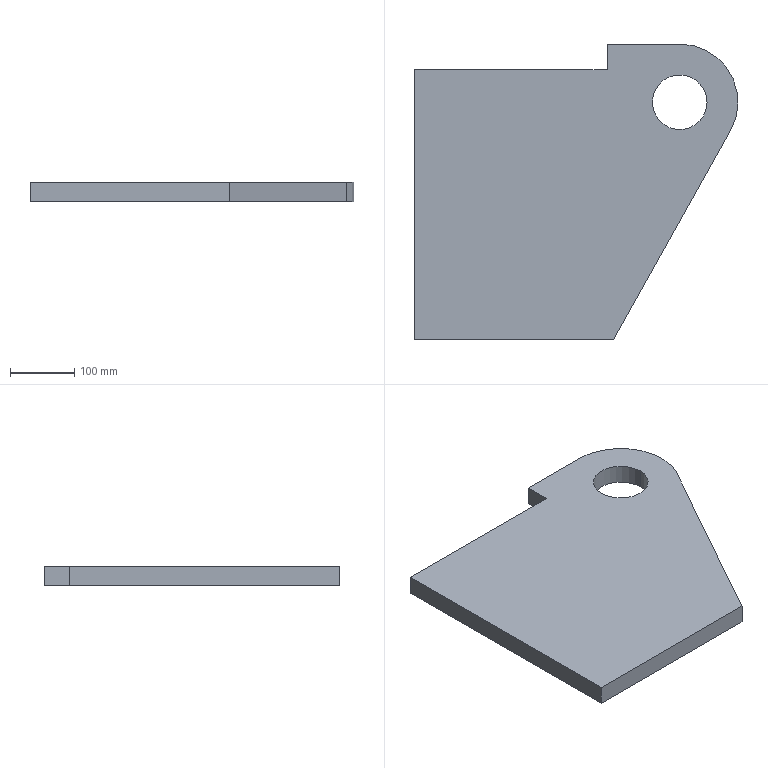Part | SolidWorks | features Extrusion 1 | 1 solid | 11 faces | box 503.5 x 460 x 30 mm | volume 5359945 mm3 | plane 8 | cylinder 3 | commonest cylinder face diameters 85 x2 181 x1
STEP:
#1=CARTESIAN_POINT('',(370.5,369.5,30.));
#2=VERTEX_POINT('',#1);
#3=CARTESIAN_POINT('',(455.5,369.5,30.));
#4=VERTEX_POINT('',#3);
#5=CARTESIAN_POINT('',(413.,369.5,30.));
#6=DIRECTION('',(0.,0.,1.));
#7=DIRECTION('',(1.,0.,0.));
#8=AXIS2_PLACEMENT_3D('',#5,#6,#7);
#9=CIRCLE('',#8,42.5);
#10=EDGE_CURVE('',#2,#4,#9,.T.);
#11=ORIENTED_EDGE('',*,*,#10,.T.);
#12=CARTESIAN_POINT('',(455.5,369.5,0.));
#13=VERTEX_POINT('',#12);
#14=CARTESIAN_POINT('',(455.5,369.5,30.));
#15=DIRECTION('',(0.,0.,-1.));
#16=VECTOR('',#15,1000.);
#17=LINE('',#14,#16);
#18=EDGE_CURVE('',#4,#13,#17,.T.);
#19=ORIENTED_EDGE('',*,*,#18,.T.);
#20=CARTESIAN_POINT('',(370.5,369.5,0.));
#21=VERTEX_POINT('',#20);
#22=CARTESIAN_POINT('',(413.,369.5,0.));
#23=DIRECTION('',(0.,0.,1.));
#24=DIRECTION('',(1.,0.,0.));
#25=AXIS2_PLACEMENT_3D('',#22,#23,#24);
#26=CIRCLE('',#25,42.5);
#27=EDGE_CURVE('',#21,#13,#26,.T.);
#28=ORIENTED_EDGE('',*,*,#27,.F.);
#29=CARTESIAN_POINT('',(370.5,369.5,30.));
#30=DIRECTION('',(0.,0.,-1.));
#31=VECTOR('',#30,1000.);
#32=LINE('',#29,#31);
#33=EDGE_CURVE('',#2,#21,#32,.T.);
#34=ORIENTED_EDGE('',*,*,#33,.F.);
#35=EDGE_LOOP('',(#11,#19,#28,#34));
#36=FACE_OUTER_BOUND('',#35,.T.);
#37=CARTESIAN_POINT('',(413.,369.5,30.));
#38=DIRECTION('',(0.,0.,-1.));
#39=DIRECTION('',(-1.,0.,0.));
#40=AXIS2_PLACEMENT_3D('',#37,#38,#39);
#41=CYLINDRICAL_SURFACE('',#40,42.5);
#42=ADVANCED_FACE('',(#36),#41,.F.);
#43=CARTESIAN_POINT('',(0.,0.,30.));
#44=VERTEX_POINT('',#43);
#45=CARTESIAN_POINT('',(310.,0.,30.));
#46=VERTEX_POINT('',#45);
#47=CARTESIAN_POINT('',(0.,0.,30.));
#48=DIRECTION('',(1.,0.,0.));
#49=VECTOR('',#48,1000.);
#50=LINE('',#47,#49);
#51=EDGE_CURVE('',#44,#46,#50,.T.);
#52=ORIENTED_EDGE('',*,*,#51,.T.);
#53=CARTESIAN_POINT('',(491.982,325.318,30.));
#54=VERTEX_POINT('',#53);
#55=CARTESIAN_POINT('',(310.,0.,30.));
#56=DIRECTION('',(0.4882,0.8727,0.));
#57=VECTOR('',#56,1000.);
#58=LINE('',#55,#57);
#59=EDGE_CURVE('',#46,#54,#58,.T.);
#60=ORIENTED_EDGE('',*,*,#59,.T.);
#61=CARTESIAN_POINT('',(413.,460.,30.));
#62=VERTEX_POINT('',#61);
#63=CARTESIAN_POINT('',(413.,369.5,30.));
#64=DIRECTION('',(0.,0.,1.));
#65=DIRECTION('',(1.,0.,0.));
#66=AXIS2_PLACEMENT_3D('',#63,#64,#65);
#67=CIRCLE('',#66,90.5);
#68=EDGE_CURVE('',#54,#62,#67,.T.);
#69=ORIENTED_EDGE('',*,*,#68,.T.);
#70=CARTESIAN_POINT('',(300.,460.,30.));
#71=VERTEX_POINT('',#70);
#72=CARTESIAN_POINT('',(300.,460.,30.));
#73=DIRECTION('',(-1.,0.,0.));
#74=VECTOR('',#73,1000.);
#75=LINE('',#72,#74);
#76=EDGE_CURVE('',#62,#71,#75,.T.);
#77=ORIENTED_EDGE('',*,*,#76,.T.);
#78=CARTESIAN_POINT('',(300.,420.,30.));
#79=VERTEX_POINT('',#78);
#80=CARTESIAN_POINT('',(300.,420.,30.));
#81=DIRECTION('',(0.,-1.,0.));
#82=VECTOR('',#81,1000.);
#83=LINE('',#80,#82);
#84=EDGE_CURVE('',#71,#79,#83,.T.);
#85=ORIENTED_EDGE('',*,*,#84,.T.);
#86=CARTESIAN_POINT('',(0.,420.,30.));
#87=VERTEX_POINT('',#86);
#88=CARTESIAN_POINT('',(0.,420.,30.));
#89=DIRECTION('',(-1.,0.,0.));
#90=VECTOR('',#89,1000.);
#91=LINE('',#88,#90);
#92=EDGE_CURVE('',#79,#87,#91,.T.);
#93=ORIENTED_EDGE('',*,*,#92,.T.);
#94=CARTESIAN_POINT('',(0.,0.,30.));
#95=DIRECTION('',(0.,-1.,0.));
#96=VECTOR('',#95,1000.);
#97=LINE('',#94,#96);
#98=EDGE_CURVE('',#87,#44,#97,.T.);
#99=ORIENTED_EDGE('',*,*,#98,.T.);
#100=EDGE_LOOP('',(#52,#60,#69,#77,#85,#93,#99));
#101=FACE_OUTER_BOUND('',#100,.T.);
#102=ORIENTED_EDGE('',*,*,#10,.F.);
#103=CARTESIAN_POINT('',(413.,369.5,30.));
#104=DIRECTION('',(0.,0.,1.));
#105=DIRECTION('',(1.,0.,0.));
#106=AXIS2_PLACEMENT_3D('',#103,#104,#105);
#107=CIRCLE('',#106,42.5);
#108=EDGE_CURVE('',#4,#2,#107,.T.);
#109=ORIENTED_EDGE('',*,*,#108,.F.);
#110=EDGE_LOOP('',(#102,#109));
#111=FACE_BOUND('',#110,.T.);
#112=CARTESIAN_POINT('',(413.,369.5,30.));
#113=DIRECTION('',(0.,0.,1.));
#114=DIRECTION('',(1.,0.,0.));
#115=AXIS2_PLACEMENT_3D('',#112,#113,#114);
#116=PLANE('',#115);
#117=ADVANCED_FACE('',(#101,#111),#116,.T.);
#118=CARTESIAN_POINT('',(0.,0.,0.));
#119=VERTEX_POINT('',#118);
#120=CARTESIAN_POINT('',(310.,0.,0.));
#121=VERTEX_POINT('',#120);
#122=CARTESIAN_POINT('',(0.,0.,0.));
#123=DIRECTION('',(1.,0.,0.));
#124=VECTOR('',#123,1000.);
#125=LINE('',#122,#124);
#126=EDGE_CURVE('',#119,#121,#125,.T.);
#127=ORIENTED_EDGE('',*,*,#126,.F.);
#128=CARTESIAN_POINT('',(0.,420.,0.));
#129=VERTEX_POINT('',#128);
#130=CARTESIAN_POINT('',(0.,0.,0.));
#131=DIRECTION('',(0.,-1.,0.));
#132=VECTOR('',#131,1000.);
#133=LINE('',#130,#132);
#134=EDGE_CURVE('',#129,#119,#133,.T.);
#135=ORIENTED_EDGE('',*,*,#134,.F.);
#136=CARTESIAN_POINT('',(300.,420.,0.));
#137=VERTEX_POINT('',#136);
#138=CARTESIAN_POINT('',(0.,420.,0.));
#139=DIRECTION('',(-1.,0.,0.));
#140=VECTOR('',#139,1000.);
#141=LINE('',#138,#140);
#142=EDGE_CURVE('',#137,#129,#141,.T.);
#143=ORIENTED_EDGE('',*,*,#142,.F.);
#144=CARTESIAN_POINT('',(300.,460.,0.));
#145=VERTEX_POINT('',#144);
#146=CARTESIAN_POINT('',(300.,420.,0.));
#147=DIRECTION('',(0.,-1.,0.));
#148=VECTOR('',#147,1000.);
#149=LINE('',#146,#148);
#150=EDGE_CURVE('',#145,#137,#149,.T.);
#151=ORIENTED_EDGE('',*,*,#150,.F.);
#152=CARTESIAN_POINT('',(413.,460.,0.));
#153=VERTEX_POINT('',#152);
#154=CARTESIAN_POINT('',(300.,460.,0.));
#155=DIRECTION('',(-1.,0.,0.));
#156=VECTOR('',#155,1000.);
#157=LINE('',#154,#156);
#158=EDGE_CURVE('',#153,#145,#157,.T.);
#159=ORIENTED_EDGE('',*,*,#158,.F.);
#160=CARTESIAN_POINT('',(491.982,325.318,0.));
#161=VERTEX_POINT('',#160);
#162=CARTESIAN_POINT('',(413.,369.5,0.));
#163=DIRECTION('',(0.,0.,1.));
#164=DIRECTION('',(1.,0.,0.));
#165=AXIS2_PLACEMENT_3D('',#162,#163,#164);
#166=CIRCLE('',#165,90.5);
#167=EDGE_CURVE('',#161,#153,#166,.T.);
#168=ORIENTED_EDGE('',*,*,#167,.F.);
#169=CARTESIAN_POINT('',(310.,0.,0.));
#170=DIRECTION('',(0.4882,0.8727,0.));
#171=VECTOR('',#170,1000.);
#172=LINE('',#169,#171);
#173=EDGE_CURVE('',#121,#161,#172,.T.);
#174=ORIENTED_EDGE('',*,*,#173,.F.);
#175=EDGE_LOOP('',(#127,#135,#143,#151,#159,#168,#174));
#176=FACE_OUTER_BOUND('',#175,.T.);
#177=ORIENTED_EDGE('',*,*,#27,.T.);
#178=CARTESIAN_POINT('',(413.,369.5,0.));
#179=DIRECTION('',(0.,0.,1.));
#180=DIRECTION('',(1.,0.,0.));
#181=AXIS2_PLACEMENT_3D('',#178,#179,#180);
#182=CIRCLE('',#181,42.5);
#183=EDGE_CURVE('',#13,#21,#182,.T.);
#184=ORIENTED_EDGE('',*,*,#183,.T.);
#185=EDGE_LOOP('',(#177,#184));
#186=FACE_BOUND('',#185,.T.);
#187=CARTESIAN_POINT('',(413.,369.5,0.));
#188=DIRECTION('',(0.,0.,1.));
#189=DIRECTION('',(1.,0.,0.));
#190=AXIS2_PLACEMENT_3D('',#187,#188,#189);
#191=PLANE('',#190);
#192=ADVANCED_FACE('',(#176,#186),#191,.F.);
#193=ORIENTED_EDGE('',*,*,#126,.T.);
#194=CARTESIAN_POINT('',(310.,0.,30.));
#195=DIRECTION('',(0.,0.,-1.));
#196=VECTOR('',#195,1000.);
#197=LINE('',#194,#196);
#198=EDGE_CURVE('',#46,#121,#197,.T.);
#199=ORIENTED_EDGE('',*,*,#198,.F.);
#200=ORIENTED_EDGE('',*,*,#51,.F.);
#201=CARTESIAN_POINT('',(0.,0.,30.));
#202=DIRECTION('',(0.,0.,-1.));
#203=VECTOR('',#202,1000.);
#204=LINE('',#201,#203);
#205=EDGE_CURVE('',#44,#119,#204,.T.);
#206=ORIENTED_EDGE('',*,*,#205,.T.);
#207=EDGE_LOOP('',(#193,#199,#200,#206));
#208=FACE_OUTER_BOUND('',#207,.T.);
#209=CARTESIAN_POINT('',(0.,0.,30.));
#210=DIRECTION('',(0.,1.,0.));
#211=DIRECTION('',(0.,0.,1.));
#212=AXIS2_PLACEMENT_3D('',#209,#210,#211);
#213=PLANE('',#212);
#214=ADVANCED_FACE('',(#208),#213,.F.);
#215=ORIENTED_EDGE('',*,*,#173,.T.);
#216=CARTESIAN_POINT('',(491.982,325.318,30.));
#217=DIRECTION('',(0.,0.,-1.));
#218=VECTOR('',#217,1000.);
#219=LINE('',#216,#218);
#220=EDGE_CURVE('',#54,#161,#219,.T.);
#221=ORIENTED_EDGE('',*,*,#220,.F.);
#222=ORIENTED_EDGE('',*,*,#59,.F.);
#223=ORIENTED_EDGE('',*,*,#198,.T.);
#224=EDGE_LOOP('',(#215,#221,#222,#223));
#225=FACE_OUTER_BOUND('',#224,.T.);
#226=CARTESIAN_POINT('',(310.,0.,30.));
#227=DIRECTION('',(-0.8727,0.4882,0.));
#228=DIRECTION('',(-0.4882,-0.8727,0.));
#229=AXIS2_PLACEMENT_3D('',#226,#227,#228);
#230=PLANE('',#229);
#231=ADVANCED_FACE('',(#225),#230,.F.);
#232=ORIENTED_EDGE('',*,*,#167,.T.);
#233=CARTESIAN_POINT('',(413.,460.,30.));
#234=DIRECTION('',(0.,0.,-1.));
#235=VECTOR('',#234,1000.);
#236=LINE('',#233,#235);
#237=EDGE_CURVE('',#62,#153,#236,.T.);
#238=ORIENTED_EDGE('',*,*,#237,.F.);
#239=ORIENTED_EDGE('',*,*,#68,.F.);
#240=ORIENTED_EDGE('',*,*,#220,.T.);
#241=EDGE_LOOP('',(#232,#238,#239,#240));
#242=FACE_OUTER_BOUND('',#241,.T.);
#243=CARTESIAN_POINT('',(413.,369.5,30.));
#244=DIRECTION('',(0.,0.,-1.));
#245=DIRECTION('',(-1.,0.,0.));
#246=AXIS2_PLACEMENT_3D('',#243,#244,#245);
#247=CYLINDRICAL_SURFACE('',#246,90.5);
#248=ADVANCED_FACE('',(#242),#247,.T.);
#249=ORIENTED_EDGE('',*,*,#158,.T.);
#250=CARTESIAN_POINT('',(300.,460.,30.));
#251=DIRECTION('',(0.,0.,-1.));
#252=VECTOR('',#251,1000.);
#253=LINE('',#250,#252);
#254=EDGE_CURVE('',#71,#145,#253,.T.);
#255=ORIENTED_EDGE('',*,*,#254,.F.);
#256=ORIENTED_EDGE('',*,*,#76,.F.);
#257=ORIENTED_EDGE('',*,*,#237,.T.);
#258=EDGE_LOOP('',(#249,#255,#256,#257));
#259=FACE_OUTER_BOUND('',#258,.T.);
#260=CARTESIAN_POINT('',(300.,460.,30.));
#261=DIRECTION('',(0.,-1.,0.));
#262=DIRECTION('',(1.,0.,0.));
#263=AXIS2_PLACEMENT_3D('',#260,#261,#262);
#264=PLANE('',#263);
#265=ADVANCED_FACE('',(#259),#264,.F.);
#266=ORIENTED_EDGE('',*,*,#150,.T.);
#267=CARTESIAN_POINT('',(300.,420.,30.));
#268=DIRECTION('',(0.,0.,-1.));
#269=VECTOR('',#268,1000.);
#270=LINE('',#267,#269);
#271=EDGE_CURVE('',#79,#137,#270,.T.);
#272=ORIENTED_EDGE('',*,*,#271,.F.);
#273=ORIENTED_EDGE('',*,*,#84,.F.);
#274=ORIENTED_EDGE('',*,*,#254,.T.);
#275=EDGE_LOOP('',(#266,#272,#273,#274));
#276=FACE_OUTER_BOUND('',#275,.T.);
#277=CARTESIAN_POINT('',(300.,420.,30.));
#278=DIRECTION('',(1.,0.,0.));
#279=DIRECTION('',(0.,0.,-1.));
#280=AXIS2_PLACEMENT_3D('',#277,#278,#279);
#281=PLANE('',#280);
#282=ADVANCED_FACE('',(#276),#281,.F.);
#283=ORIENTED_EDGE('',*,*,#142,.T.);
#284=CARTESIAN_POINT('',(0.,420.,30.));
#285=DIRECTION('',(0.,0.,-1.));
#286=VECTOR('',#285,1000.);
#287=LINE('',#284,#286);
#288=EDGE_CURVE('',#87,#129,#287,.T.);
#289=ORIENTED_EDGE('',*,*,#288,.F.);
#290=ORIENTED_EDGE('',*,*,#92,.F.);
#291=ORIENTED_EDGE('',*,*,#271,.T.);
#292=EDGE_LOOP('',(#283,#289,#290,#291));
#293=FACE_OUTER_BOUND('',#292,.T.);
#294=CARTESIAN_POINT('',(0.,420.,30.));
#295=DIRECTION('',(0.,-1.,0.));
#296=DIRECTION('',(0.,0.,-1.));
#297=AXIS2_PLACEMENT_3D('',#294,#295,#296);
#298=PLANE('',#297);
#299=ADVANCED_FACE('',(#293),#298,.F.);
#300=ORIENTED_EDGE('',*,*,#134,.T.);
#301=ORIENTED_EDGE('',*,*,#205,.F.);
#302=ORIENTED_EDGE('',*,*,#98,.F.);
#303=ORIENTED_EDGE('',*,*,#288,.T.);
#304=EDGE_LOOP('',(#300,#301,#302,#303));
#305=FACE_OUTER_BOUND('',#304,.T.);
#306=CARTESIAN_POINT('',(0.,0.,30.));
#307=DIRECTION('',(1.,0.,0.));
#308=DIRECTION('',(0.,0.,-1.));
#309=AXIS2_PLACEMENT_3D('',#306,#307,#308);
#310=PLANE('',#309);
#311=ADVANCED_FACE('',(#305),#310,.F.);
#312=ORIENTED_EDGE('',*,*,#18,.F.);
#313=ORIENTED_EDGE('',*,*,#108,.T.);
#314=ORIENTED_EDGE('',*,*,#33,.T.);
#315=ORIENTED_EDGE('',*,*,#183,.F.);
#316=EDGE_LOOP('',(#312,#313,#314,#315));
#317=FACE_OUTER_BOUND('',#316,.T.);
#318=CARTESIAN_POINT('',(413.,369.5,30.));
#319=DIRECTION('',(0.,0.,-1.));
#320=DIRECTION('',(-1.,0.,0.));
#321=AXIS2_PLACEMENT_3D('',#318,#319,#320);
#322=CYLINDRICAL_SURFACE('',#321,42.5);
#323=ADVANCED_FACE('',(#317),#322,.F.);
#324=CLOSED_SHELL('',(#42,#117,#192,#214,#231,#248,#265,#282,#299,#311,#323));
#325=MANIFOLD_SOLID_BREP('',#324);
#326=CARTESIAN_POINT('',(0.,0.,0.));
#327=DIRECTION('',(0.,0.,1.));
#328=DIRECTION('',(1.,0.,0.));
#329=AXIS2_PLACEMENT_3D('',#326,#327,#328);
#330=(LENGTH_UNIT()NAMED_UNIT(*)SI_UNIT(.MILLI.,.METRE.));
#331=UNCERTAINTY_MEASURE_WITH_UNIT(LENGTH_MEASURE(0.00001),#330,'','');
#332=(NAMED_UNIT(*)PLANE_ANGLE_UNIT()SI_UNIT($,.RADIAN.));
#333=(NAMED_UNIT(*)SI_UNIT($,.STERADIAN.)SOLID_ANGLE_UNIT());
#334=(GEOMETRIC_REPRESENTATION_CONTEXT(3)GLOBAL_UNCERTAINTY_ASSIGNED_CONTEXT((#331))GLOBAL_UNIT_ASSIGNED_CONTEXT((#330,#332,#333))REPRESENTATION_CONTEXT('',''));
#335=ADVANCED_BREP_SHAPE_REPRESENTATION('',(#325,#329),#334);